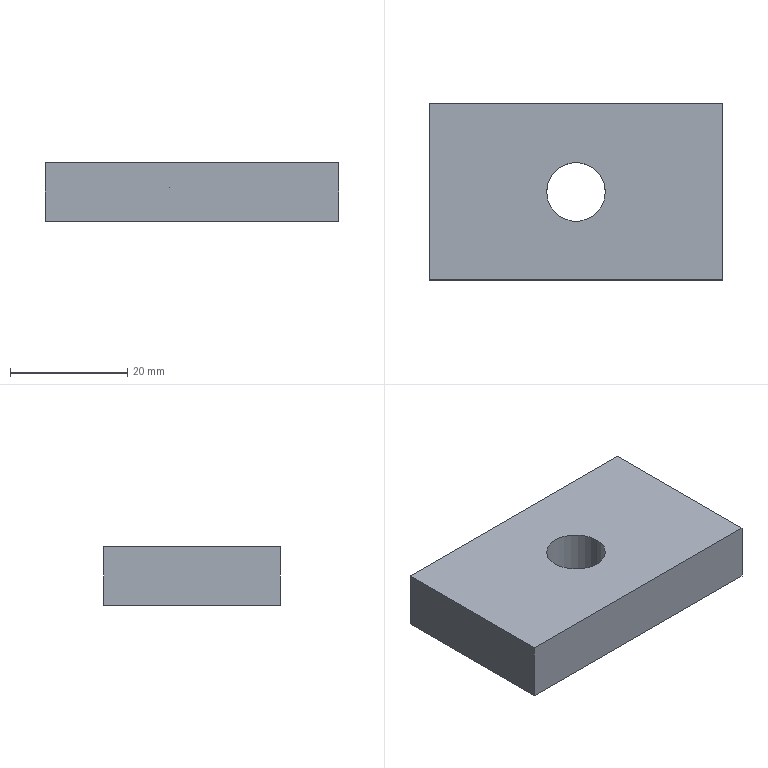Part | SolidWorks | features Extrusion 1 | 1 solid | 8 faces | box 50 x 30 x 10 mm | volume 14215 mm3 | plane 6 | cylinder 2 | commonest cylinder face diameters 10 x2
STEP:
#1=CARTESIAN_POINT('',(-5.,0.,-5.));
#2=VERTEX_POINT('',#1);
#3=CARTESIAN_POINT('',(5.,0.,-5.));
#4=VERTEX_POINT('',#3);
#5=CARTESIAN_POINT('',(0.,0.,-5.));
#6=DIRECTION('',(0.,0.,1.));
#7=DIRECTION('',(-1.,0.,0.));
#8=AXIS2_PLACEMENT_3D('',#5,#6,#7);
#9=CIRCLE('',#8,5.);
#10=EDGE_CURVE('',#2,#4,#9,.T.);
#11=ORIENTED_EDGE('',*,*,#10,.F.);
#12=CARTESIAN_POINT('',(-5.,0.,5.));
#13=VERTEX_POINT('',#12);
#14=CARTESIAN_POINT('',(-5.,0.,-5.));
#15=DIRECTION('',(0.,0.,1.));
#16=VECTOR('',#15,1000.);
#17=LINE('',#14,#16);
#18=EDGE_CURVE('',#2,#13,#17,.T.);
#19=ORIENTED_EDGE('',*,*,#18,.T.);
#20=CARTESIAN_POINT('',(5.,0.,5.));
#21=VERTEX_POINT('',#20);
#22=CARTESIAN_POINT('',(0.,0.,5.));
#23=DIRECTION('',(0.,0.,1.));
#24=DIRECTION('',(-1.,0.,0.));
#25=AXIS2_PLACEMENT_3D('',#22,#23,#24);
#26=CIRCLE('',#25,5.);
#27=EDGE_CURVE('',#13,#21,#26,.T.);
#28=ORIENTED_EDGE('',*,*,#27,.T.);
#29=CARTESIAN_POINT('',(5.,0.,-5.));
#30=DIRECTION('',(0.,0.,1.));
#31=VECTOR('',#30,1000.);
#32=LINE('',#29,#31);
#33=EDGE_CURVE('',#4,#21,#32,.T.);
#34=ORIENTED_EDGE('',*,*,#33,.F.);
#35=EDGE_LOOP('',(#11,#19,#28,#34));
#36=FACE_OUTER_BOUND('',#35,.T.);
#37=CARTESIAN_POINT('',(0.,0.,-5.));
#38=DIRECTION('',(0.,0.,1.));
#39=DIRECTION('',(1.,0.,0.));
#40=AXIS2_PLACEMENT_3D('',#37,#38,#39);
#41=CYLINDRICAL_SURFACE('',#40,5.);
#42=ADVANCED_FACE('',(#36),#41,.F.);
#43=CARTESIAN_POINT('',(25.,15.,5.));
#44=VERTEX_POINT('',#43);
#45=CARTESIAN_POINT('',(-25.,15.,5.));
#46=VERTEX_POINT('',#45);
#47=CARTESIAN_POINT('',(25.,15.,5.));
#48=DIRECTION('',(-1.,0.,0.));
#49=VECTOR('',#48,1000.);
#50=LINE('',#47,#49);
#51=EDGE_CURVE('',#44,#46,#50,.T.);
#52=ORIENTED_EDGE('',*,*,#51,.F.);
#53=CARTESIAN_POINT('',(25.,15.,-5.));
#54=VERTEX_POINT('',#53);
#55=CARTESIAN_POINT('',(25.,15.,-5.));
#56=DIRECTION('',(0.,0.,1.));
#57=VECTOR('',#56,1000.);
#58=LINE('',#55,#57);
#59=EDGE_CURVE('',#54,#44,#58,.T.);
#60=ORIENTED_EDGE('',*,*,#59,.F.);
#61=CARTESIAN_POINT('',(-25.,15.,-5.));
#62=VERTEX_POINT('',#61);
#63=CARTESIAN_POINT('',(25.,15.,-5.));
#64=DIRECTION('',(-1.,0.,0.));
#65=VECTOR('',#64,1000.);
#66=LINE('',#63,#65);
#67=EDGE_CURVE('',#54,#62,#66,.T.);
#68=ORIENTED_EDGE('',*,*,#67,.T.);
#69=CARTESIAN_POINT('',(-25.,15.,-5.));
#70=DIRECTION('',(0.,0.,1.));
#71=VECTOR('',#70,1000.);
#72=LINE('',#69,#71);
#73=EDGE_CURVE('',#62,#46,#72,.T.);
#74=ORIENTED_EDGE('',*,*,#73,.T.);
#75=EDGE_LOOP('',(#52,#60,#68,#74));
#76=FACE_OUTER_BOUND('',#75,.T.);
#77=CARTESIAN_POINT('',(25.,15.,-5.));
#78=DIRECTION('',(0.,1.,0.));
#79=DIRECTION('',(0.,0.,1.));
#80=AXIS2_PLACEMENT_3D('',#77,#78,#79);
#81=PLANE('',#80);
#82=ADVANCED_FACE('',(#76),#81,.T.);
#83=CARTESIAN_POINT('',(25.,-15.,5.));
#84=VERTEX_POINT('',#83);
#85=CARTESIAN_POINT('',(25.,-15.,5.));
#86=DIRECTION('',(0.,1.,0.));
#87=VECTOR('',#86,1000.);
#88=LINE('',#85,#87);
#89=EDGE_CURVE('',#84,#44,#88,.T.);
#90=ORIENTED_EDGE('',*,*,#89,.F.);
#91=CARTESIAN_POINT('',(25.,-15.,-5.));
#92=VERTEX_POINT('',#91);
#93=CARTESIAN_POINT('',(25.,-15.,-5.));
#94=DIRECTION('',(0.,0.,1.));
#95=VECTOR('',#94,1000.);
#96=LINE('',#93,#95);
#97=EDGE_CURVE('',#92,#84,#96,.T.);
#98=ORIENTED_EDGE('',*,*,#97,.F.);
#99=CARTESIAN_POINT('',(25.,-15.,-5.));
#100=DIRECTION('',(0.,1.,0.));
#101=VECTOR('',#100,1000.);
#102=LINE('',#99,#101);
#103=EDGE_CURVE('',#92,#54,#102,.T.);
#104=ORIENTED_EDGE('',*,*,#103,.T.);
#105=ORIENTED_EDGE('',*,*,#59,.T.);
#106=EDGE_LOOP('',(#90,#98,#104,#105));
#107=FACE_OUTER_BOUND('',#106,.T.);
#108=CARTESIAN_POINT('',(25.,-15.,-5.));
#109=DIRECTION('',(1.,0.,0.));
#110=DIRECTION('',(0.,0.,-1.));
#111=AXIS2_PLACEMENT_3D('',#108,#109,#110);
#112=PLANE('',#111);
#113=ADVANCED_FACE('',(#107),#112,.T.);
#114=CARTESIAN_POINT('',(-25.,-15.,5.));
#115=VERTEX_POINT('',#114);
#116=CARTESIAN_POINT('',(-25.,-15.,5.));
#117=DIRECTION('',(1.,0.,0.));
#118=VECTOR('',#117,1000.);
#119=LINE('',#116,#118);
#120=EDGE_CURVE('',#115,#84,#119,.T.);
#121=ORIENTED_EDGE('',*,*,#120,.F.);
#122=CARTESIAN_POINT('',(-25.,-15.,-5.));
#123=VERTEX_POINT('',#122);
#124=CARTESIAN_POINT('',(-25.,-15.,-5.));
#125=DIRECTION('',(0.,0.,1.));
#126=VECTOR('',#125,1000.);
#127=LINE('',#124,#126);
#128=EDGE_CURVE('',#123,#115,#127,.T.);
#129=ORIENTED_EDGE('',*,*,#128,.F.);
#130=CARTESIAN_POINT('',(-25.,-15.,-5.));
#131=DIRECTION('',(1.,0.,0.));
#132=VECTOR('',#131,1000.);
#133=LINE('',#130,#132);
#134=EDGE_CURVE('',#123,#92,#133,.T.);
#135=ORIENTED_EDGE('',*,*,#134,.T.);
#136=ORIENTED_EDGE('',*,*,#97,.T.);
#137=EDGE_LOOP('',(#121,#129,#135,#136));
#138=FACE_OUTER_BOUND('',#137,.T.);
#139=CARTESIAN_POINT('',(-25.,-15.,-5.));
#140=DIRECTION('',(0.,-1.,0.));
#141=DIRECTION('',(0.,0.,-1.));
#142=AXIS2_PLACEMENT_3D('',#139,#140,#141);
#143=PLANE('',#142);
#144=ADVANCED_FACE('',(#138),#143,.T.);
#145=CARTESIAN_POINT('',(-25.,15.,5.));
#146=DIRECTION('',(0.,-1.,0.));
#147=VECTOR('',#146,1000.);
#148=LINE('',#145,#147);
#149=EDGE_CURVE('',#46,#115,#148,.T.);
#150=ORIENTED_EDGE('',*,*,#149,.F.);
#151=ORIENTED_EDGE('',*,*,#73,.F.);
#152=CARTESIAN_POINT('',(-25.,15.,-5.));
#153=DIRECTION('',(0.,-1.,0.));
#154=VECTOR('',#153,1000.);
#155=LINE('',#152,#154);
#156=EDGE_CURVE('',#62,#123,#155,.T.);
#157=ORIENTED_EDGE('',*,*,#156,.T.);
#158=ORIENTED_EDGE('',*,*,#128,.T.);
#159=EDGE_LOOP('',(#150,#151,#157,#158));
#160=FACE_OUTER_BOUND('',#159,.T.);
#161=CARTESIAN_POINT('',(-25.,15.,-5.));
#162=DIRECTION('',(-1.,0.,0.));
#163=DIRECTION('',(0.,0.,1.));
#164=AXIS2_PLACEMENT_3D('',#161,#162,#163);
#165=PLANE('',#164);
#166=ADVANCED_FACE('',(#160),#165,.T.);
#167=CARTESIAN_POINT('',(0.,0.,-5.));
#168=DIRECTION('',(0.,0.,1.));
#169=DIRECTION('',(-1.,0.,0.));
#170=AXIS2_PLACEMENT_3D('',#167,#168,#169);
#171=CIRCLE('',#170,5.);
#172=EDGE_CURVE('',#4,#2,#171,.T.);
#173=ORIENTED_EDGE('',*,*,#172,.T.);
#174=ORIENTED_EDGE('',*,*,#10,.T.);
#175=EDGE_LOOP('',(#173,#174));
#176=FACE_BOUND('',#175,.T.);
#177=ORIENTED_EDGE('',*,*,#67,.F.);
#178=ORIENTED_EDGE('',*,*,#103,.F.);
#179=ORIENTED_EDGE('',*,*,#134,.F.);
#180=ORIENTED_EDGE('',*,*,#156,.F.);
#181=EDGE_LOOP('',(#177,#178,#179,#180));
#182=FACE_OUTER_BOUND('',#181,.T.);
#183=CARTESIAN_POINT('',(0.,0.,-5.));
#184=DIRECTION('',(0.,0.,1.));
#185=DIRECTION('',(1.,0.,0.));
#186=AXIS2_PLACEMENT_3D('',#183,#184,#185);
#187=PLANE('',#186);
#188=ADVANCED_FACE('',(#176,#182),#187,.F.);
#189=CARTESIAN_POINT('',(0.,0.,5.));
#190=DIRECTION('',(0.,0.,1.));
#191=DIRECTION('',(-1.,0.,0.));
#192=AXIS2_PLACEMENT_3D('',#189,#190,#191);
#193=CIRCLE('',#192,5.);
#194=EDGE_CURVE('',#21,#13,#193,.T.);
#195=ORIENTED_EDGE('',*,*,#194,.F.);
#196=ORIENTED_EDGE('',*,*,#27,.F.);
#197=EDGE_LOOP('',(#195,#196));
#198=FACE_BOUND('',#197,.T.);
#199=ORIENTED_EDGE('',*,*,#51,.T.);
#200=ORIENTED_EDGE('',*,*,#149,.T.);
#201=ORIENTED_EDGE('',*,*,#120,.T.);
#202=ORIENTED_EDGE('',*,*,#89,.T.);
#203=EDGE_LOOP('',(#199,#200,#201,#202));
#204=FACE_OUTER_BOUND('',#203,.T.);
#205=CARTESIAN_POINT('',(0.,0.,5.));
#206=DIRECTION('',(0.,0.,1.));
#207=DIRECTION('',(1.,0.,0.));
#208=AXIS2_PLACEMENT_3D('',#205,#206,#207);
#209=PLANE('',#208);
#210=ADVANCED_FACE('',(#198,#204),#209,.T.);
#211=ORIENTED_EDGE('',*,*,#18,.F.);
#212=ORIENTED_EDGE('',*,*,#172,.F.);
#213=ORIENTED_EDGE('',*,*,#33,.T.);
#214=ORIENTED_EDGE('',*,*,#194,.T.);
#215=EDGE_LOOP('',(#211,#212,#213,#214));
#216=FACE_OUTER_BOUND('',#215,.T.);
#217=CARTESIAN_POINT('',(0.,0.,-5.));
#218=DIRECTION('',(0.,0.,1.));
#219=DIRECTION('',(1.,0.,0.));
#220=AXIS2_PLACEMENT_3D('',#217,#218,#219);
#221=CYLINDRICAL_SURFACE('',#220,5.);
#222=ADVANCED_FACE('',(#216),#221,.F.);
#223=CLOSED_SHELL('',(#42,#82,#113,#144,#166,#188,#210,#222));
#224=MANIFOLD_SOLID_BREP('',#223);
#225=CARTESIAN_POINT('',(0.,0.,0.));
#226=DIRECTION('',(0.,0.,1.));
#227=DIRECTION('',(1.,0.,0.));
#228=AXIS2_PLACEMENT_3D('',#225,#226,#227);
#229=(LENGTH_UNIT()NAMED_UNIT(*)SI_UNIT(.MILLI.,.METRE.));
#230=UNCERTAINTY_MEASURE_WITH_UNIT(LENGTH_MEASURE(0.00001),#229,'','');
#231=(NAMED_UNIT(*)PLANE_ANGLE_UNIT()SI_UNIT($,.RADIAN.));
#232=(NAMED_UNIT(*)SI_UNIT($,.STERADIAN.)SOLID_ANGLE_UNIT());
#233=(GEOMETRIC_REPRESENTATION_CONTEXT(3)GLOBAL_UNCERTAINTY_ASSIGNED_CONTEXT((#230))GLOBAL_UNIT_ASSIGNED_CONTEXT((#229,#231,#232))REPRESENTATION_CONTEXT('',''));
#234=ADVANCED_BREP_SHAPE_REPRESENTATION('',(#224,#228),#233);